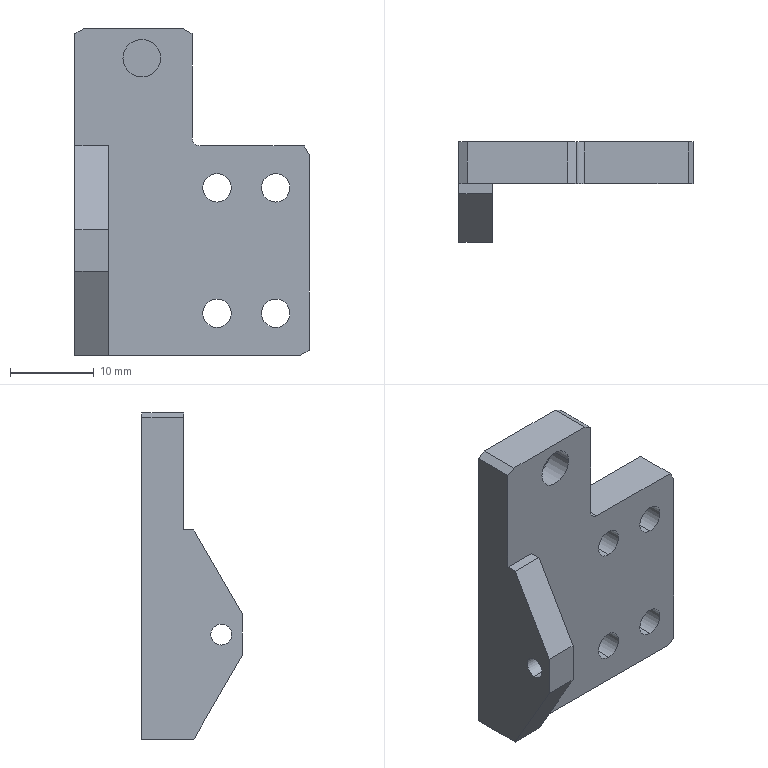Part | NX | features BREP 1 | 1 solid | 39 faces | box 28 x 12 x 39 mm | volume 4638 mm3 | plane 18 | cylinder 13 | cone 8 | commonest cylinder face diameters 3.4 x8 2.5 x2 4.5 x2 2 x1
STEP:
#1=CARTESIAN_POINT('',(14.,12.,13.5));
#2=VERTEX_POINT('',#1);
#3=CARTESIAN_POINT('',(15.,12.,12.5));
#4=VERTEX_POINT('',#3);
#5=CARTESIAN_POINT('',(15.,12.,13.5));
#6=DIRECTION('',(0.,-1.,0.));
#7=DIRECTION('',(0.,0.,-1.));
#8=AXIS2_PLACEMENT_3D('',#5,#6,#7);
#9=CIRCLE('',#8,1.);
#10=EDGE_CURVE('',#2,#4,#9,.T.);
#11=ORIENTED_EDGE('',*,*,#10,.F.);
#12=CARTESIAN_POINT('',(14.,7.,13.5));
#13=VERTEX_POINT('',#12);
#14=CARTESIAN_POINT('',(14.,12.,13.5));
#15=DIRECTION('',(0.,1.,0.));
#16=VECTOR('',#15,1000.);
#17=LINE('',#14,#16);
#18=EDGE_CURVE('',#13,#2,#17,.T.);
#19=ORIENTED_EDGE('',*,*,#18,.F.);
#20=CARTESIAN_POINT('',(15.,7.,12.5));
#21=VERTEX_POINT('',#20);
#22=CARTESIAN_POINT('',(15.,7.,13.5));
#23=DIRECTION('',(0.,1.,0.));
#24=DIRECTION('',(-1.,0.,0.));
#25=AXIS2_PLACEMENT_3D('',#22,#23,#24);
#26=CIRCLE('',#25,1.);
#27=EDGE_CURVE('',#21,#13,#26,.T.);
#28=ORIENTED_EDGE('',*,*,#27,.F.);
#29=CARTESIAN_POINT('',(15.,0.,12.5));
#30=DIRECTION('',(0.,-1.,0.));
#31=VECTOR('',#30,1000.);
#32=LINE('',#29,#31);
#33=EDGE_CURVE('',#4,#21,#32,.T.);
#34=ORIENTED_EDGE('',*,*,#33,.F.);
#35=EDGE_LOOP('',(#11,#19,#28,#34));
#36=FACE_BOUND('',#35,.T.);
#37=CARTESIAN_POINT('',(15.,0.,13.5));
#38=DIRECTION('',(0.,-1.,0.));
#39=DIRECTION('',(1.,0.,0.));
#40=AXIS2_PLACEMENT_3D('',#37,#38,#39);
#41=CYLINDRICAL_SURFACE('',#40,1.);
#42=ADVANCED_FACE('',(#36),#41,.F.);
#43=CARTESIAN_POINT('',(13.,12.,26.5));
#44=VERTEX_POINT('',#43);
#45=CARTESIAN_POINT('',(14.,12.,25.923));
#46=VERTEX_POINT('',#45);
#47=CARTESIAN_POINT('',(14.,12.,25.923));
#48=DIRECTION('',(0.866,0.,-0.5));
#49=VECTOR('',#48,1000.);
#50=LINE('',#47,#49);
#51=EDGE_CURVE('',#44,#46,#50,.T.);
#52=ORIENTED_EDGE('',*,*,#51,.F.);
#53=CARTESIAN_POINT('',(13.,7.,26.5));
#54=VERTEX_POINT('',#53);
#55=CARTESIAN_POINT('',(13.,0.,26.5));
#56=DIRECTION('',(0.,1.,0.));
#57=VECTOR('',#56,1000.);
#58=LINE('',#55,#57);
#59=EDGE_CURVE('',#54,#44,#58,.T.);
#60=ORIENTED_EDGE('',*,*,#59,.F.);
#61=CARTESIAN_POINT('',(14.,7.,25.923));
#62=VERTEX_POINT('',#61);
#63=CARTESIAN_POINT('',(14.,7.,25.923));
#64=DIRECTION('',(-0.866,0.,0.5));
#65=VECTOR('',#64,1000.);
#66=LINE('',#63,#65);
#67=EDGE_CURVE('',#62,#54,#66,.T.);
#68=ORIENTED_EDGE('',*,*,#67,.F.);
#69=CARTESIAN_POINT('',(14.,12.,25.923));
#70=DIRECTION('',(0.,-1.,0.));
#71=VECTOR('',#70,1000.);
#72=LINE('',#69,#71);
#73=EDGE_CURVE('',#46,#62,#72,.T.);
#74=ORIENTED_EDGE('',*,*,#73,.F.);
#75=EDGE_LOOP('',(#52,#60,#68,#74));
#76=FACE_BOUND('',#75,.T.);
#77=CARTESIAN_POINT('',(14.,12.,25.923));
#78=DIRECTION('',(-0.5,0.,-0.866));
#79=DIRECTION('',(0.,-1.,0.));
#80=AXIS2_PLACEMENT_3D('',#77,#78,#79);
#81=PLANE('',#80);
#82=ADVANCED_FACE('',(#76),#81,.F.);
#83=CARTESIAN_POINT('',(1.,7.,26.5));
#84=VERTEX_POINT('',#83);
#85=CARTESIAN_POINT('',(0.,7.,25.923));
#86=VERTEX_POINT('',#85);
#87=CARTESIAN_POINT('',(0.,7.,25.923));
#88=DIRECTION('',(-0.866,0.,-0.5));
#89=VECTOR('',#88,1000.);
#90=LINE('',#87,#89);
#91=EDGE_CURVE('',#84,#86,#90,.T.);
#92=ORIENTED_EDGE('',*,*,#91,.F.);
#93=CARTESIAN_POINT('',(1.,12.,26.5));
#94=VERTEX_POINT('',#93);
#95=CARTESIAN_POINT('',(1.,7.,26.5));
#96=DIRECTION('',(0.,-1.,0.));
#97=VECTOR('',#96,1000.);
#98=LINE('',#95,#97);
#99=EDGE_CURVE('',#94,#84,#98,.T.);
#100=ORIENTED_EDGE('',*,*,#99,.F.);
#101=CARTESIAN_POINT('',(0.,12.,25.923));
#102=VERTEX_POINT('',#101);
#103=CARTESIAN_POINT('',(0.,12.,25.923));
#104=DIRECTION('',(0.866,0.,0.5));
#105=VECTOR('',#104,1000.);
#106=LINE('',#103,#105);
#107=EDGE_CURVE('',#102,#94,#106,.T.);
#108=ORIENTED_EDGE('',*,*,#107,.F.);
#109=CARTESIAN_POINT('',(0.,12.,25.923));
#110=DIRECTION('',(0.,1.,0.));
#111=VECTOR('',#110,1000.);
#112=LINE('',#109,#111);
#113=EDGE_CURVE('',#86,#102,#112,.T.);
#114=ORIENTED_EDGE('',*,*,#113,.F.);
#115=EDGE_LOOP('',(#92,#100,#108,#114));
#116=FACE_BOUND('',#115,.T.);
#117=CARTESIAN_POINT('',(0.,0.,25.923));
#118=DIRECTION('',(-0.5,0.,0.866));
#119=DIRECTION('',(0.,-1.,0.));
#120=AXIS2_PLACEMENT_3D('',#117,#118,#119);
#121=PLANE('',#120);
#122=ADVANCED_FACE('',(#116),#121,.T.);
#123=CARTESIAN_POINT('',(27.,7.,-12.5));
#124=VERTEX_POINT('',#123);
#125=CARTESIAN_POINT('',(28.,7.,-11.923));
#126=VERTEX_POINT('',#125);
#127=CARTESIAN_POINT('',(28.,7.,-11.923));
#128=DIRECTION('',(0.866,0.,0.5));
#129=VECTOR('',#128,1000.);
#130=LINE('',#127,#129);
#131=EDGE_CURVE('',#124,#126,#130,.T.);
#132=ORIENTED_EDGE('',*,*,#131,.F.);
#133=CARTESIAN_POINT('',(27.,12.,-12.5));
#134=VERTEX_POINT('',#133);
#135=CARTESIAN_POINT('',(27.,7.,-12.5));
#136=DIRECTION('',(0.,-1.,0.));
#137=VECTOR('',#136,1000.);
#138=LINE('',#135,#137);
#139=EDGE_CURVE('',#134,#124,#138,.T.);
#140=ORIENTED_EDGE('',*,*,#139,.F.);
#141=CARTESIAN_POINT('',(28.,12.,-11.923));
#142=VERTEX_POINT('',#141);
#143=CARTESIAN_POINT('',(28.,12.,-11.923));
#144=DIRECTION('',(-0.866,0.,-0.5));
#145=VECTOR('',#144,1000.);
#146=LINE('',#143,#145);
#147=EDGE_CURVE('',#142,#134,#146,.T.);
#148=ORIENTED_EDGE('',*,*,#147,.F.);
#149=CARTESIAN_POINT('',(28.,12.,-11.923));
#150=DIRECTION('',(0.,1.,0.));
#151=VECTOR('',#150,1000.);
#152=LINE('',#149,#151);
#153=EDGE_CURVE('',#126,#142,#152,.T.);
#154=ORIENTED_EDGE('',*,*,#153,.F.);
#155=EDGE_LOOP('',(#132,#140,#148,#154));
#156=FACE_BOUND('',#155,.T.);
#157=CARTESIAN_POINT('',(28.,12.,-11.923));
#158=DIRECTION('',(0.5,0.,-0.866));
#159=DIRECTION('',(0.,-1.,0.));
#160=AXIS2_PLACEMENT_3D('',#157,#158,#159);
#161=PLANE('',#160);
#162=ADVANCED_FACE('',(#156),#161,.T.);
#163=CARTESIAN_POINT('',(28.,7.,11.5));
#164=VERTEX_POINT('',#163);
#165=CARTESIAN_POINT('',(27.423,7.,12.5));
#166=VERTEX_POINT('',#165);
#167=CARTESIAN_POINT('',(27.423,7.,12.5));
#168=DIRECTION('',(-0.5,0.,0.866));
#169=VECTOR('',#168,1000.);
#170=LINE('',#167,#169);
#171=EDGE_CURVE('',#164,#166,#170,.T.);
#172=ORIENTED_EDGE('',*,*,#171,.F.);
#173=CARTESIAN_POINT('',(28.,12.,11.5));
#174=VERTEX_POINT('',#173);
#175=CARTESIAN_POINT('',(28.,12.,11.5));
#176=DIRECTION('',(0.,-1.,0.));
#177=VECTOR('',#176,1000.);
#178=LINE('',#175,#177);
#179=EDGE_CURVE('',#174,#164,#178,.T.);
#180=ORIENTED_EDGE('',*,*,#179,.F.);
#181=CARTESIAN_POINT('',(27.423,12.,12.5));
#182=VERTEX_POINT('',#181);
#183=CARTESIAN_POINT('',(27.423,12.,12.5));
#184=DIRECTION('',(0.5,0.,-0.866));
#185=VECTOR('',#184,1000.);
#186=LINE('',#183,#185);
#187=EDGE_CURVE('',#182,#174,#186,.T.);
#188=ORIENTED_EDGE('',*,*,#187,.F.);
#189=CARTESIAN_POINT('',(27.423,0.,12.5));
#190=DIRECTION('',(0.,1.,0.));
#191=VECTOR('',#190,1000.);
#192=LINE('',#189,#191);
#193=EDGE_CURVE('',#166,#182,#192,.T.);
#194=ORIENTED_EDGE('',*,*,#193,.F.);
#195=EDGE_LOOP('',(#172,#180,#188,#194));
#196=FACE_BOUND('',#195,.T.);
#197=CARTESIAN_POINT('',(27.423,0.,12.5));
#198=DIRECTION('',(-0.866,0.,-0.5));
#199=DIRECTION('',(0.,1.,0.));
#200=AXIS2_PLACEMENT_3D('',#197,#198,#199);
#201=PLANE('',#200);
#202=ADVANCED_FACE('',(#196),#201,.F.);
#203=CARTESIAN_POINT('',(10.25,10.,23.));
#204=VERTEX_POINT('',#203);
#205=CARTESIAN_POINT('',(5.75,10.,23.));
#206=VERTEX_POINT('',#205);
#207=CARTESIAN_POINT('',(8.,10.,23.));
#208=DIRECTION('',(0.,-1.,0.));
#209=DIRECTION('',(1.,0.,0.));
#210=AXIS2_PLACEMENT_3D('',#207,#208,#209);
#211=CIRCLE('',#210,2.25);
#212=EDGE_CURVE('',#204,#206,#211,.T.);
#213=ORIENTED_EDGE('',*,*,#212,.T.);
#214=CARTESIAN_POINT('',(8.,10.,23.));
#215=DIRECTION('',(0.,-1.,0.));
#216=DIRECTION('',(1.,0.,0.));
#217=AXIS2_PLACEMENT_3D('',#214,#215,#216);
#218=CIRCLE('',#217,2.25);
#219=EDGE_CURVE('',#206,#204,#218,.T.);
#220=ORIENTED_EDGE('',*,*,#219,.T.);
#221=EDGE_LOOP('',(#213,#220));
#222=FACE_BOUND('',#221,.T.);
#223=CARTESIAN_POINT('',(8.,10.,23.));
#224=DIRECTION('',(0.,-1.,0.));
#225=DIRECTION('',(1.,0.,0.));
#226=AXIS2_PLACEMENT_3D('',#223,#224,#225);
#227=PLANE('',#226);
#228=ADVANCED_FACE('',(#222),#227,.T.);
#229=CARTESIAN_POINT('',(5.75,7.,23.));
#230=VERTEX_POINT('',#229);
#231=CARTESIAN_POINT('',(5.75,10.,23.));
#232=DIRECTION('',(0.,-1.,0.));
#233=VECTOR('',#232,1000.);
#234=LINE('',#231,#233);
#235=EDGE_CURVE('',#230,#206,#234,.F.);
#236=ORIENTED_EDGE('',*,*,#235,.T.);
#237=ORIENTED_EDGE('',*,*,#212,.F.);
#238=CARTESIAN_POINT('',(10.25,7.,23.));
#239=VERTEX_POINT('',#238);
#240=CARTESIAN_POINT('',(10.25,10.,23.));
#241=DIRECTION('',(0.,-1.,0.));
#242=VECTOR('',#241,1000.);
#243=LINE('',#240,#242);
#244=EDGE_CURVE('',#239,#204,#243,.F.);
#245=ORIENTED_EDGE('',*,*,#244,.F.);
#246=CARTESIAN_POINT('',(8.,7.,23.));
#247=DIRECTION('',(0.,-1.,0.));
#248=DIRECTION('',(1.,0.,0.));
#249=AXIS2_PLACEMENT_3D('',#246,#247,#248);
#250=CIRCLE('',#249,2.25);
#251=EDGE_CURVE('',#239,#230,#250,.T.);
#252=ORIENTED_EDGE('',*,*,#251,.T.);
#253=EDGE_LOOP('',(#236,#237,#245,#252));
#254=FACE_BOUND('',#253,.T.);
#255=CARTESIAN_POINT('',(8.,10.,23.));
#256=DIRECTION('',(0.,-1.,0.));
#257=DIRECTION('',(1.,0.,0.));
#258=AXIS2_PLACEMENT_3D('',#255,#256,#257);
#259=CYLINDRICAL_SURFACE('',#258,2.25);
#260=ADVANCED_FACE('',(#254),#259,.F.);
#261=CARTESIAN_POINT('',(0.,12.,26.5));
#262=DIRECTION('',(1.,0.,0.));
#263=VECTOR('',#262,1000.);
#264=LINE('',#261,#263);
#265=EDGE_CURVE('',#94,#44,#264,.T.);
#266=ORIENTED_EDGE('',*,*,#265,.F.);
#267=ORIENTED_EDGE('',*,*,#99,.T.);
#268=CARTESIAN_POINT('',(0.,7.,26.5));
#269=DIRECTION('',(-1.,0.,0.));
#270=VECTOR('',#269,1000.);
#271=LINE('',#268,#270);
#272=EDGE_CURVE('',#54,#84,#271,.T.);
#273=ORIENTED_EDGE('',*,*,#272,.F.);
#274=ORIENTED_EDGE('',*,*,#59,.T.);
#275=EDGE_LOOP('',(#266,#267,#273,#274));
#276=FACE_BOUND('',#275,.T.);
#277=CARTESIAN_POINT('',(0.,0.,26.5));
#278=DIRECTION('',(0.,0.,1.));
#279=DIRECTION('',(1.,0.,0.));
#280=AXIS2_PLACEMENT_3D('',#277,#278,#279);
#281=PLANE('',#280);
#282=ADVANCED_FACE('',(#276),#281,.T.);
#283=CARTESIAN_POINT('',(14.,7.,26.5));
#284=DIRECTION('',(0.,0.,-1.));
#285=VECTOR('',#284,1000.);
#286=LINE('',#283,#285);
#287=EDGE_CURVE('',#62,#13,#286,.T.);
#288=ORIENTED_EDGE('',*,*,#287,.T.);
#289=ORIENTED_EDGE('',*,*,#18,.T.);
#290=CARTESIAN_POINT('',(14.,12.,26.5));
#291=DIRECTION('',(0.,0.,-1.));
#292=VECTOR('',#291,1000.);
#293=LINE('',#290,#292);
#294=EDGE_CURVE('',#46,#2,#293,.T.);
#295=ORIENTED_EDGE('',*,*,#294,.F.);
#296=ORIENTED_EDGE('',*,*,#73,.T.);
#297=EDGE_LOOP('',(#288,#289,#295,#296));
#298=FACE_BOUND('',#297,.T.);
#299=CARTESIAN_POINT('',(14.,12.,26.5));
#300=DIRECTION('',(1.,0.,0.));
#301=DIRECTION('',(0.,1.,0.));
#302=AXIS2_PLACEMENT_3D('',#299,#300,#301);
#303=PLANE('',#302);
#304=ADVANCED_FACE('',(#298),#303,.T.);
#305=CARTESIAN_POINT('',(0.,0.,2.5));
#306=VERTEX_POINT('',#305);
#307=CARTESIAN_POINT('',(0.,5.774,12.5));
#308=VERTEX_POINT('',#307);
#309=CARTESIAN_POINT('',(0.,5.774,12.5));
#310=DIRECTION('',(0.,0.5,0.866));
#311=VECTOR('',#310,1000.);
#312=LINE('',#309,#311);
#313=EDGE_CURVE('',#306,#308,#312,.T.);
#314=ORIENTED_EDGE('',*,*,#313,.F.);
#315=CARTESIAN_POINT('',(4.,0.,2.5));
#316=VERTEX_POINT('',#315);
#317=CARTESIAN_POINT('',(4.,0.,2.5));
#318=DIRECTION('',(-1.,0.,0.));
#319=VECTOR('',#318,1000.);
#320=LINE('',#317,#319);
#321=EDGE_CURVE('',#316,#306,#320,.T.);
#322=ORIENTED_EDGE('',*,*,#321,.F.);
#323=CARTESIAN_POINT('',(4.,5.774,12.5));
#324=VERTEX_POINT('',#323);
#325=CARTESIAN_POINT('',(4.,5.774,12.5));
#326=DIRECTION('',(0.,-0.5,-0.866));
#327=VECTOR('',#326,1000.);
#328=LINE('',#325,#327);
#329=EDGE_CURVE('',#324,#316,#328,.T.);
#330=ORIENTED_EDGE('',*,*,#329,.F.);
#331=CARTESIAN_POINT('',(0.,5.774,12.5));
#332=DIRECTION('',(1.,0.,0.));
#333=VECTOR('',#332,1000.);
#334=LINE('',#331,#333);
#335=EDGE_CURVE('',#308,#324,#334,.T.);
#336=ORIENTED_EDGE('',*,*,#335,.F.);
#337=EDGE_LOOP('',(#314,#322,#330,#336));
#338=FACE_BOUND('',#337,.T.);
#339=CARTESIAN_POINT('',(0.,5.774,12.5));
#340=DIRECTION('',(0.,0.866,-0.5));
#341=DIRECTION('',(1.,0.,0.));
#342=AXIS2_PLACEMENT_3D('',#339,#340,#341);
#343=PLANE('',#342);
#344=ADVANCED_FACE('',(#338),#343,.F.);
#345=CARTESIAN_POINT('',(0.,5.774,-12.5));
#346=VERTEX_POINT('',#345);
#347=CARTESIAN_POINT('',(0.,0.,-2.5));
#348=VERTEX_POINT('',#347);
#349=CARTESIAN_POINT('',(0.,0.,-2.5));
#350=DIRECTION('',(0.,-0.5,0.866));
#351=VECTOR('',#350,1000.);
#352=LINE('',#349,#351);
#353=EDGE_CURVE('',#346,#348,#352,.T.);
#354=ORIENTED_EDGE('',*,*,#353,.F.);
#355=CARTESIAN_POINT('',(4.,5.774,-12.5));
#356=VERTEX_POINT('',#355);
#357=CARTESIAN_POINT('',(0.,5.774,-12.5));
#358=DIRECTION('',(-1.,0.,0.));
#359=VECTOR('',#358,1000.);
#360=LINE('',#357,#359);
#361=EDGE_CURVE('',#356,#346,#360,.T.);
#362=ORIENTED_EDGE('',*,*,#361,.F.);
#363=CARTESIAN_POINT('',(4.,0.,-2.5));
#364=VERTEX_POINT('',#363);
#365=CARTESIAN_POINT('',(4.,0.,-2.5));
#366=DIRECTION('',(0.,0.5,-0.866));
#367=VECTOR('',#366,1000.);
#368=LINE('',#365,#367);
#369=EDGE_CURVE('',#364,#356,#368,.T.);
#370=ORIENTED_EDGE('',*,*,#369,.F.);
#371=CARTESIAN_POINT('',(4.,0.,-2.5));
#372=DIRECTION('',(1.,0.,0.));
#373=VECTOR('',#372,1000.);
#374=LINE('',#371,#373);
#375=EDGE_CURVE('',#348,#364,#374,.T.);
#376=ORIENTED_EDGE('',*,*,#375,.F.);
#377=EDGE_LOOP('',(#354,#362,#370,#376));
#378=FACE_BOUND('',#377,.T.);
#379=CARTESIAN_POINT('',(4.,0.,-2.5));
#380=DIRECTION('',(0.,-0.866,-0.5));
#381=DIRECTION('',(-1.,0.,0.));
#382=AXIS2_PLACEMENT_3D('',#379,#380,#381);
#383=PLANE('',#382);
#384=ADVANCED_FACE('',(#378),#383,.T.);
#385=CARTESIAN_POINT('',(17.,12.,4.35));
#386=VERTEX_POINT('',#385);
#387=CARTESIAN_POINT('',(17.,10.55,5.8));
#388=VERTEX_POINT('',#387);
#389=CARTESIAN_POINT('',(17.,12.,4.35));
#390=DIRECTION('',(0.,0.7071,-0.7071));
#391=VECTOR('',#390,1000.);
#392=LINE('',#389,#391);
#393=EDGE_CURVE('',#386,#388,#392,.F.);
#394=ORIENTED_EDGE('',*,*,#393,.T.);
#395=CARTESIAN_POINT('',(17.,10.55,9.2));
#396=VERTEX_POINT('',#395);
#397=CARTESIAN_POINT('',(17.,10.55,7.5));
#398=DIRECTION('',(0.,1.,0.));
#399=DIRECTION('',(0.,0.,1.));
#400=AXIS2_PLACEMENT_3D('',#397,#398,#399);
#401=CIRCLE('',#400,1.7);
#402=EDGE_CURVE('',#396,#388,#401,.T.);
#403=ORIENTED_EDGE('',*,*,#402,.F.);
#404=CARTESIAN_POINT('',(17.,12.,10.65));
#405=VERTEX_POINT('',#404);
#406=CARTESIAN_POINT('',(17.,12.,10.65));
#407=DIRECTION('',(0.,0.7071,0.7071));
#408=VECTOR('',#407,1000.);
#409=LINE('',#406,#408);
#410=EDGE_CURVE('',#405,#396,#409,.F.);
#411=ORIENTED_EDGE('',*,*,#410,.F.);
#412=CARTESIAN_POINT('',(17.,12.,7.5));
#413=DIRECTION('',(0.,1.,0.));
#414=DIRECTION('',(0.,0.,1.));
#415=AXIS2_PLACEMENT_3D('',#412,#413,#414);
#416=CIRCLE('',#415,3.15);
#417=EDGE_CURVE('',#405,#386,#416,.T.);
#418=ORIENTED_EDGE('',*,*,#417,.T.);
#419=EDGE_LOOP('',(#394,#403,#411,#418));
#420=FACE_BOUND('',#419,.T.);
#421=CARTESIAN_POINT('',(17.,12.,7.5));
#422=DIRECTION('',(0.,1.,0.));
#423=DIRECTION('',(0.,0.,1.));
#424=AXIS2_PLACEMENT_3D('',#421,#422,#423);
#425=CONICAL_SURFACE('',#424,3.15,0.7854);
#426=ADVANCED_FACE('',(#420),#425,.F.);
#427=CARTESIAN_POINT('',(17.,7.,5.8));
#428=VERTEX_POINT('',#427);
#429=CARTESIAN_POINT('',(17.,12.,5.8));
#430=DIRECTION('',(0.,1.,0.));
#431=VECTOR('',#430,1000.);
#432=LINE('',#429,#431);
#433=EDGE_CURVE('',#388,#428,#432,.F.);
#434=ORIENTED_EDGE('',*,*,#433,.T.);
#435=CARTESIAN_POINT('',(17.,7.,9.2));
#436=VERTEX_POINT('',#435);
#437=CARTESIAN_POINT('',(17.,7.,7.5));
#438=DIRECTION('',(0.,1.,0.));
#439=DIRECTION('',(-1.,0.,0.));
#440=AXIS2_PLACEMENT_3D('',#437,#438,#439);
#441=CIRCLE('',#440,1.7);
#442=EDGE_CURVE('',#436,#428,#441,.T.);
#443=ORIENTED_EDGE('',*,*,#442,.F.);
#444=CARTESIAN_POINT('',(17.,12.,9.2));
#445=DIRECTION('',(0.,1.,0.));
#446=VECTOR('',#445,1000.);
#447=LINE('',#444,#446);
#448=EDGE_CURVE('',#396,#436,#447,.F.);
#449=ORIENTED_EDGE('',*,*,#448,.F.);
#450=ORIENTED_EDGE('',*,*,#402,.T.);
#451=EDGE_LOOP('',(#434,#443,#449,#450));
#452=FACE_BOUND('',#451,.T.);
#453=CARTESIAN_POINT('',(17.,12.,7.5));
#454=DIRECTION('',(0.,1.,0.));
#455=DIRECTION('',(0.,0.,1.));
#456=AXIS2_PLACEMENT_3D('',#453,#454,#455);
#457=CYLINDRICAL_SURFACE('',#456,1.7);
#458=ADVANCED_FACE('',(#452),#457,.F.);
#459=CARTESIAN_POINT('',(24.,12.,4.35));
#460=VERTEX_POINT('',#459);
#461=CARTESIAN_POINT('',(24.,10.55,5.8));
#462=VERTEX_POINT('',#461);
#463=CARTESIAN_POINT('',(24.,12.,4.35));
#464=DIRECTION('',(0.,0.7071,-0.7071));
#465=VECTOR('',#464,1000.);
#466=LINE('',#463,#465);
#467=EDGE_CURVE('',#460,#462,#466,.F.);
#468=ORIENTED_EDGE('',*,*,#467,.T.);
#469=CARTESIAN_POINT('',(24.,10.55,9.2));
#470=VERTEX_POINT('',#469);
#471=CARTESIAN_POINT('',(24.,10.55,7.5));
#472=DIRECTION('',(0.,1.,0.));
#473=DIRECTION('',(0.,0.,1.));
#474=AXIS2_PLACEMENT_3D('',#471,#472,#473);
#475=CIRCLE('',#474,1.7);
#476=EDGE_CURVE('',#470,#462,#475,.T.);
#477=ORIENTED_EDGE('',*,*,#476,.F.);
#478=CARTESIAN_POINT('',(24.,12.,10.65));
#479=VERTEX_POINT('',#478);
#480=CARTESIAN_POINT('',(24.,12.,10.65));
#481=DIRECTION('',(0.,0.7071,0.7071));
#482=VECTOR('',#481,1000.);
#483=LINE('',#480,#482);
#484=EDGE_CURVE('',#479,#470,#483,.F.);
#485=ORIENTED_EDGE('',*,*,#484,.F.);
#486=CARTESIAN_POINT('',(24.,12.,7.5));
#487=DIRECTION('',(0.,1.,0.));
#488=DIRECTION('',(0.,0.,1.));
#489=AXIS2_PLACEMENT_3D('',#486,#487,#488);
#490=CIRCLE('',#489,3.15);
#491=EDGE_CURVE('',#479,#460,#490,.T.);
#492=ORIENTED_EDGE('',*,*,#491,.T.);
#493=EDGE_LOOP('',(#468,#477,#485,#492));
#494=FACE_BOUND('',#493,.T.);
#495=CARTESIAN_POINT('',(24.,12.,7.5));
#496=DIRECTION('',(0.,1.,0.));
#497=DIRECTION('',(0.,0.,1.));
#498=AXIS2_PLACEMENT_3D('',#495,#496,#497);
#499=CONICAL_SURFACE('',#498,3.15,0.7854);
#500=ADVANCED_FACE('',(#494),#499,.F.);
#501=CARTESIAN_POINT('',(24.,7.,5.8));
#502=VERTEX_POINT('',#501);
#503=CARTESIAN_POINT('',(24.,12.,5.8));
#504=DIRECTION('',(0.,1.,0.));
#505=VECTOR('',#504,1000.);
#506=LINE('',#503,#505);
#507=EDGE_CURVE('',#462,#502,#506,.F.);
#508=ORIENTED_EDGE('',*,*,#507,.T.);
#509=CARTESIAN_POINT('',(24.,7.,9.2));
#510=VERTEX_POINT('',#509);
#511=CARTESIAN_POINT('',(24.,7.,7.5));
#512=DIRECTION('',(0.,1.,0.));
#513=DIRECTION('',(-1.,0.,0.));
#514=AXIS2_PLACEMENT_3D('',#511,#512,#513);
#515=CIRCLE('',#514,1.7);
#516=EDGE_CURVE('',#510,#502,#515,.T.);
#517=ORIENTED_EDGE('',*,*,#516,.F.);
#518=CARTESIAN_POINT('',(24.,12.,9.2));
#519=DIRECTION('',(0.,1.,0.));
#520=VECTOR('',#519,1000.);
#521=LINE('',#518,#520);
#522=EDGE_CURVE('',#470,#510,#521,.F.);
#523=ORIENTED_EDGE('',*,*,#522,.F.);
#524=ORIENTED_EDGE('',*,*,#476,.T.);
#525=EDGE_LOOP('',(#508,#517,#523,#524));
#526=FACE_BOUND('',#525,.T.);
#527=CARTESIAN_POINT('',(24.,12.,7.5));
#528=DIRECTION('',(0.,1.,0.));
#529=DIRECTION('',(0.,0.,1.));
#530=AXIS2_PLACEMENT_3D('',#527,#528,#529);
#531=CYLINDRICAL_SURFACE('',#530,1.7);
#532=ADVANCED_FACE('',(#526),#531,.F.);
#533=CARTESIAN_POINT('',(17.,12.,-10.65));
#534=VERTEX_POINT('',#533);
#535=CARTESIAN_POINT('',(17.,10.55,-9.2));
#536=VERTEX_POINT('',#535);
#537=CARTESIAN_POINT('',(17.,12.,-10.65));
#538=DIRECTION('',(0.,0.7071,-0.7071));
#539=VECTOR('',#538,1000.);
#540=LINE('',#537,#539);
#541=EDGE_CURVE('',#534,#536,#540,.F.);
#542=ORIENTED_EDGE('',*,*,#541,.T.);
#543=CARTESIAN_POINT('',(17.,10.55,-5.8));
#544=VERTEX_POINT('',#543);
#545=CARTESIAN_POINT('',(17.,10.55,-7.5));
#546=DIRECTION('',(0.,1.,0.));
#547=DIRECTION('',(0.,0.,1.));
#548=AXIS2_PLACEMENT_3D('',#545,#546,#547);
#549=CIRCLE('',#548,1.7);
#550=EDGE_CURVE('',#544,#536,#549,.T.);
#551=ORIENTED_EDGE('',*,*,#550,.F.);
#552=CARTESIAN_POINT('',(17.,12.,-4.35));
#553=VERTEX_POINT('',#552);
#554=CARTESIAN_POINT('',(17.,12.,-4.35));
#555=DIRECTION('',(0.,0.7071,0.7071));
#556=VECTOR('',#555,1000.);
#557=LINE('',#554,#556);
#558=EDGE_CURVE('',#553,#544,#557,.F.);
#559=ORIENTED_EDGE('',*,*,#558,.F.);
#560=CARTESIAN_POINT('',(17.,12.,-7.5));
#561=DIRECTION('',(0.,1.,0.));
#562=DIRECTION('',(0.,0.,1.));
#563=AXIS2_PLACEMENT_3D('',#560,#561,#562);
#564=CIRCLE('',#563,3.15);
#565=EDGE_CURVE('',#553,#534,#564,.T.);
#566=ORIENTED_EDGE('',*,*,#565,.T.);
#567=EDGE_LOOP('',(#542,#551,#559,#566));
#568=FACE_BOUND('',#567,.T.);
#569=CARTESIAN_POINT('',(17.,12.,-7.5));
#570=DIRECTION('',(0.,1.,0.));
#571=DIRECTION('',(0.,0.,1.));
#572=AXIS2_PLACEMENT_3D('',#569,#570,#571);
#573=CONICAL_SURFACE('',#572,3.15,0.7854);
#574=ADVANCED_FACE('',(#568),#573,.F.);
#575=CARTESIAN_POINT('',(17.,7.,-9.2));
#576=VERTEX_POINT('',#575);
#577=CARTESIAN_POINT('',(17.,12.,-9.2));
#578=DIRECTION('',(0.,1.,0.));
#579=VECTOR('',#578,1000.);
#580=LINE('',#577,#579);
#581=EDGE_CURVE('',#536,#576,#580,.F.);
#582=ORIENTED_EDGE('',*,*,#581,.T.);
#583=CARTESIAN_POINT('',(17.,7.,-5.8));
#584=VERTEX_POINT('',#583);
#585=CARTESIAN_POINT('',(17.,7.,-7.5));
#586=DIRECTION('',(0.,1.,0.));
#587=DIRECTION('',(-1.,0.,0.));
#588=AXIS2_PLACEMENT_3D('',#585,#586,#587);
#589=CIRCLE('',#588,1.7);
#590=EDGE_CURVE('',#584,#576,#589,.T.);
#591=ORIENTED_EDGE('',*,*,#590,.F.);
#592=CARTESIAN_POINT('',(17.,12.,-5.8));
#593=DIRECTION('',(0.,1.,0.));
#594=VECTOR('',#593,1000.);
#595=LINE('',#592,#594);
#596=EDGE_CURVE('',#544,#584,#595,.F.);
#597=ORIENTED_EDGE('',*,*,#596,.F.);
#598=ORIENTED_EDGE('',*,*,#550,.T.);
#599=EDGE_LOOP('',(#582,#591,#597,#598));
#600=FACE_BOUND('',#599,.T.);
#601=CARTESIAN_POINT('',(17.,12.,-7.5));
#602=DIRECTION('',(0.,1.,0.));
#603=DIRECTION('',(0.,0.,1.));
#604=AXIS2_PLACEMENT_3D('',#601,#602,#603);
#605=CYLINDRICAL_SURFACE('',#604,1.7);
#606=ADVANCED_FACE('',(#600),#605,.F.);
#607=CARTESIAN_POINT('',(24.,12.,-10.65));
#608=VERTEX_POINT('',#607);
#609=CARTESIAN_POINT('',(24.,10.55,-9.2));
#610=VERTEX_POINT('',#609);
#611=CARTESIAN_POINT('',(24.,12.,-10.65));
#612=DIRECTION('',(0.,0.7071,-0.7071));
#613=VECTOR('',#612,1000.);
#614=LINE('',#611,#613);
#615=EDGE_CURVE('',#608,#610,#614,.F.);
#616=ORIENTED_EDGE('',*,*,#615,.T.);
#617=CARTESIAN_POINT('',(24.,10.55,-5.8));
#618=VERTEX_POINT('',#617);
#619=CARTESIAN_POINT('',(24.,10.55,-7.5));
#620=DIRECTION('',(0.,1.,0.));
#621=DIRECTION('',(0.,0.,1.));
#622=AXIS2_PLACEMENT_3D('',#619,#620,#621);
#623=CIRCLE('',#622,1.7);
#624=EDGE_CURVE('',#618,#610,#623,.T.);
#625=ORIENTED_EDGE('',*,*,#624,.F.);
#626=CARTESIAN_POINT('',(24.,12.,-4.35));
#627=VERTEX_POINT('',#626);
#628=CARTESIAN_POINT('',(24.,12.,-4.35));
#629=DIRECTION('',(0.,0.7071,0.7071));
#630=VECTOR('',#629,1000.);
#631=LINE('',#628,#630);
#632=EDGE_CURVE('',#627,#618,#631,.F.);
#633=ORIENTED_EDGE('',*,*,#632,.F.);
#634=CARTESIAN_POINT('',(24.,12.,-7.5));
#635=DIRECTION('',(0.,1.,0.));
#636=DIRECTION('',(0.,0.,1.));
#637=AXIS2_PLACEMENT_3D('',#634,#635,#636);
#638=CIRCLE('',#637,3.15);
#639=EDGE_CURVE('',#627,#608,#638,.T.);
#640=ORIENTED_EDGE('',*,*,#639,.T.);
#641=EDGE_LOOP('',(#616,#625,#633,#640));
#642=FACE_BOUND('',#641,.T.);
#643=CARTESIAN_POINT('',(24.,12.,-7.5));
#644=DIRECTION('',(0.,1.,0.));
#645=DIRECTION('',(0.,0.,1.));
#646=AXIS2_PLACEMENT_3D('',#643,#644,#645);
#647=CONICAL_SURFACE('',#646,3.15,0.7854);
#648=ADVANCED_FACE('',(#642),#647,.F.);
#649=CARTESIAN_POINT('',(24.,7.,-9.2));
#650=VERTEX_POINT('',#649);
#651=CARTESIAN_POINT('',(24.,12.,-9.2));
#652=DIRECTION('',(0.,1.,0.));
#653=VECTOR('',#652,1000.);
#654=LINE('',#651,#653);
#655=EDGE_CURVE('',#610,#650,#654,.F.);
#656=ORIENTED_EDGE('',*,*,#655,.T.);
#657=CARTESIAN_POINT('',(24.,7.,-5.8));
#658=VERTEX_POINT('',#657);
#659=CARTESIAN_POINT('',(24.,7.,-7.5));
#660=DIRECTION('',(0.,1.,0.));
#661=DIRECTION('',(-1.,0.,0.));
#662=AXIS2_PLACEMENT_3D('',#659,#660,#661);
#663=CIRCLE('',#662,1.7);
#664=EDGE_CURVE('',#658,#650,#663,.T.);
#665=ORIENTED_EDGE('',*,*,#664,.F.);
#666=CARTESIAN_POINT('',(24.,12.,-5.8));
#667=DIRECTION('',(0.,1.,0.));
#668=VECTOR('',#667,1000.);
#669=LINE('',#666,#668);
#670=EDGE_CURVE('',#618,#658,#669,.F.);
#671=ORIENTED_EDGE('',*,*,#670,.F.);
#672=ORIENTED_EDGE('',*,*,#624,.T.);
#673=EDGE_LOOP('',(#656,#665,#671,#672));
#674=FACE_BOUND('',#673,.T.);
#675=CARTESIAN_POINT('',(24.,12.,-7.5));
#676=DIRECTION('',(0.,1.,0.));
#677=DIRECTION('',(0.,0.,1.));
#678=AXIS2_PLACEMENT_3D('',#675,#676,#677);
#679=CYLINDRICAL_SURFACE('',#678,1.7);
#680=ADVANCED_FACE('',(#674),#679,.F.);
#681=CARTESIAN_POINT('',(0.,2.5,-1.25));
#682=VERTEX_POINT('',#681);
#683=CARTESIAN_POINT('',(4.,2.5,-1.25));
#684=VERTEX_POINT('',#683);
#685=CARTESIAN_POINT('',(0.,2.5,-1.25));
#686=DIRECTION('',(-1.,0.,0.));
#687=VECTOR('',#686,1000.);
#688=LINE('',#685,#687);
#689=EDGE_CURVE('',#682,#684,#688,.F.);
#690=ORIENTED_EDGE('',*,*,#689,.T.);
#691=CARTESIAN_POINT('',(4.,2.5,1.25));
#692=VERTEX_POINT('',#691);
#693=CARTESIAN_POINT('',(4.,2.5,0.));
#694=DIRECTION('',(-1.,0.,0.));
#695=DIRECTION('',(0.,0.,1.));
#696=AXIS2_PLACEMENT_3D('',#693,#694,#695);
#697=CIRCLE('',#696,1.25);
#698=EDGE_CURVE('',#692,#684,#697,.T.);
#699=ORIENTED_EDGE('',*,*,#698,.F.);
#700=CARTESIAN_POINT('',(0.,2.5,1.25));
#701=VERTEX_POINT('',#700);
#702=CARTESIAN_POINT('',(0.,2.5,1.25));
#703=DIRECTION('',(-1.,0.,0.));
#704=VECTOR('',#703,1000.);
#705=LINE('',#702,#704);
#706=EDGE_CURVE('',#701,#692,#705,.F.);
#707=ORIENTED_EDGE('',*,*,#706,.F.);
#708=CARTESIAN_POINT('',(0.,2.5,0.));
#709=DIRECTION('',(-1.,0.,0.));
#710=DIRECTION('',(0.,0.,1.));
#711=AXIS2_PLACEMENT_3D('',#708,#709,#710);
#712=CIRCLE('',#711,1.25);
#713=EDGE_CURVE('',#701,#682,#712,.T.);
#714=ORIENTED_EDGE('',*,*,#713,.T.);
#715=EDGE_LOOP('',(#690,#699,#707,#714));
#716=FACE_BOUND('',#715,.T.);
#717=CARTESIAN_POINT('',(0.,2.5,0.));
#718=DIRECTION('',(-1.,0.,0.));
#719=DIRECTION('',(0.,0.,1.));
#720=AXIS2_PLACEMENT_3D('',#717,#718,#719);
#721=CYLINDRICAL_SURFACE('',#720,1.25);
#722=ADVANCED_FACE('',(#716),#721,.F.);
#723=CARTESIAN_POINT('',(0.,12.,-12.5));
#724=VERTEX_POINT('',#723);
#725=CARTESIAN_POINT('',(0.,12.,-12.5));
#726=DIRECTION('',(-1.,0.,0.));
#727=VECTOR('',#726,1000.);
#728=LINE('',#725,#727);
#729=EDGE_CURVE('',#134,#724,#728,.T.);
#730=ORIENTED_EDGE('',*,*,#729,.F.);
#731=ORIENTED_EDGE('',*,*,#139,.T.);
#732=CARTESIAN_POINT('',(4.,7.,-12.5));
#733=VERTEX_POINT('',#732);
#734=CARTESIAN_POINT('',(28.,7.,-12.5));
#735=DIRECTION('',(1.,0.,0.));
#736=VECTOR('',#735,1000.);
#737=LINE('',#734,#736);
#738=EDGE_CURVE('',#733,#124,#737,.T.);
#739=ORIENTED_EDGE('',*,*,#738,.F.);
#740=CARTESIAN_POINT('',(4.,7.,-12.5));
#741=DIRECTION('',(0.,1.,0.));
#742=VECTOR('',#741,1000.);
#743=LINE('',#740,#742);
#744=EDGE_CURVE('',#356,#733,#743,.T.);
#745=ORIENTED_EDGE('',*,*,#744,.F.);
#746=ORIENTED_EDGE('',*,*,#361,.T.);
#747=CARTESIAN_POINT('',(0.,0.,-12.5));
#748=DIRECTION('',(0.,-1.,0.));
#749=VECTOR('',#748,1000.);
#750=LINE('',#747,#749);
#751=EDGE_CURVE('',#724,#346,#750,.T.);
#752=ORIENTED_EDGE('',*,*,#751,.F.);
#753=EDGE_LOOP('',(#730,#731,#739,#745,#746,#752));
#754=FACE_BOUND('',#753,.T.);
#755=CARTESIAN_POINT('',(0.,0.,-12.5));
#756=DIRECTION('',(0.,0.,-1.));
#757=DIRECTION('',(-1.,0.,0.));
#758=AXIS2_PLACEMENT_3D('',#755,#756,#757);
#759=PLANE('',#758);
#760=ADVANCED_FACE('',(#754),#759,.T.);
#761=CARTESIAN_POINT('',(4.,7.,12.5));
#762=VERTEX_POINT('',#761);
#763=CARTESIAN_POINT('',(4.,7.,12.5));
#764=DIRECTION('',(0.,1.,0.));
#765=VECTOR('',#764,1000.);
#766=LINE('',#763,#765);
#767=EDGE_CURVE('',#324,#762,#766,.T.);
#768=ORIENTED_EDGE('',*,*,#767,.T.);
#769=CARTESIAN_POINT('',(0.,7.,12.5));
#770=VERTEX_POINT('',#769);
#771=CARTESIAN_POINT('',(0.,7.,12.5));
#772=DIRECTION('',(-1.,0.,0.));
#773=VECTOR('',#772,1000.);
#774=LINE('',#771,#773);
#775=EDGE_CURVE('',#762,#770,#774,.T.);
#776=ORIENTED_EDGE('',*,*,#775,.T.);
#777=CARTESIAN_POINT('',(0.,0.,12.5));
#778=DIRECTION('',(0.,-1.,0.));
#779=VECTOR('',#778,1000.);
#780=LINE('',#777,#779);
#781=EDGE_CURVE('',#770,#308,#780,.T.);
#782=ORIENTED_EDGE('',*,*,#781,.T.);
#783=ORIENTED_EDGE('',*,*,#335,.T.);
#784=EDGE_LOOP('',(#768,#776,#782,#783));
#785=FACE_BOUND('',#784,.T.);
#786=CARTESIAN_POINT('',(0.,0.,12.5));
#787=DIRECTION('',(0.,0.,-1.));
#788=DIRECTION('',(-1.,0.,0.));
#789=AXIS2_PLACEMENT_3D('',#786,#787,#788);
#790=PLANE('',#789);
#791=ADVANCED_FACE('',(#785),#790,.F.);
#792=CARTESIAN_POINT('',(0.,7.,26.5));
#793=DIRECTION('',(0.,0.,-1.));
#794=VECTOR('',#793,1000.);
#795=LINE('',#792,#794);
#796=EDGE_CURVE('',#86,#770,#795,.T.);
#797=ORIENTED_EDGE('',*,*,#796,.F.);
#798=ORIENTED_EDGE('',*,*,#113,.T.);
#799=CARTESIAN_POINT('',(0.,12.,12.5));
#800=DIRECTION('',(0.,0.,-1.));
#801=VECTOR('',#800,1000.);
#802=LINE('',#799,#801);
#803=EDGE_CURVE('',#102,#724,#802,.T.);
#804=ORIENTED_EDGE('',*,*,#803,.T.);
#805=ORIENTED_EDGE('',*,*,#751,.T.);
#806=ORIENTED_EDGE('',*,*,#353,.T.);
#807=CARTESIAN_POINT('',(0.,0.,12.5));
#808=DIRECTION('',(0.,0.,-1.));
#809=VECTOR('',#808,1000.);
#810=LINE('',#807,#809);
#811=EDGE_CURVE('',#306,#348,#810,.T.);
#812=ORIENTED_EDGE('',*,*,#811,.F.);
#813=ORIENTED_EDGE('',*,*,#313,.T.);
#814=ORIENTED_EDGE('',*,*,#781,.F.);
#815=EDGE_LOOP('',(#797,#798,#804,#805,#806,#812,#813,#814));
#816=FACE_BOUND('',#815,.T.);
#817=ORIENTED_EDGE('',*,*,#713,.F.);
#818=CARTESIAN_POINT('',(0.,2.5,0.));
#819=DIRECTION('',(-1.,0.,0.));
#820=DIRECTION('',(0.,0.,1.));
#821=AXIS2_PLACEMENT_3D('',#818,#819,#820);
#822=CIRCLE('',#821,1.25);
#823=EDGE_CURVE('',#682,#701,#822,.T.);
#824=ORIENTED_EDGE('',*,*,#823,.F.);
#825=EDGE_LOOP('',(#817,#824));
#826=FACE_BOUND('',#825,.T.);
#827=CARTESIAN_POINT('',(0.,0.,12.5));
#828=DIRECTION('',(1.,0.,0.));
#829=DIRECTION('',(0.,0.,-1.));
#830=AXIS2_PLACEMENT_3D('',#827,#828,#829);
#831=PLANE('',#830);
#832=ADVANCED_FACE('',(#816,#826),#831,.F.);
#833=CARTESIAN_POINT('',(0.,12.,12.5));
#834=DIRECTION('',(-1.,0.,0.));
#835=VECTOR('',#834,1000.);
#836=LINE('',#833,#835);
#837=EDGE_CURVE('',#182,#4,#836,.T.);
#838=ORIENTED_EDGE('',*,*,#837,.F.);
#839=ORIENTED_EDGE('',*,*,#187,.T.);
#840=CARTESIAN_POINT('',(28.,12.,12.5));
#841=DIRECTION('',(0.,0.,-1.));
#842=VECTOR('',#841,1000.);
#843=LINE('',#840,#842);
#844=EDGE_CURVE('',#174,#142,#843,.T.);
#845=ORIENTED_EDGE('',*,*,#844,.T.);
#846=ORIENTED_EDGE('',*,*,#147,.T.);
#847=ORIENTED_EDGE('',*,*,#729,.T.);
#848=ORIENTED_EDGE('',*,*,#803,.F.);
#849=ORIENTED_EDGE('',*,*,#107,.T.);
#850=ORIENTED_EDGE('',*,*,#265,.T.);
#851=ORIENTED_EDGE('',*,*,#51,.T.);
#852=ORIENTED_EDGE('',*,*,#294,.T.);
#853=ORIENTED_EDGE('',*,*,#10,.T.);
#854=EDGE_LOOP('',(#838,#839,#845,#846,#847,#848,#849,#850,#851,#852,#853));
#855=FACE_BOUND('',#854,.T.);
#856=ORIENTED_EDGE('',*,*,#639,.F.);
#857=CARTESIAN_POINT('',(24.,12.,-7.5));
#858=DIRECTION('',(0.,1.,0.));
#859=DIRECTION('',(0.,0.,1.));
#860=AXIS2_PLACEMENT_3D('',#857,#858,#859);
#861=CIRCLE('',#860,3.15);
#862=EDGE_CURVE('',#608,#627,#861,.T.);
#863=ORIENTED_EDGE('',*,*,#862,.F.);
#864=EDGE_LOOP('',(#856,#863));
#865=FACE_BOUND('',#864,.T.);
#866=ORIENTED_EDGE('',*,*,#565,.F.);
#867=CARTESIAN_POINT('',(17.,12.,-7.5));
#868=DIRECTION('',(0.,1.,0.));
#869=DIRECTION('',(0.,0.,1.));
#870=AXIS2_PLACEMENT_3D('',#867,#868,#869);
#871=CIRCLE('',#870,3.15);
#872=EDGE_CURVE('',#534,#553,#871,.T.);
#873=ORIENTED_EDGE('',*,*,#872,.F.);
#874=EDGE_LOOP('',(#866,#873));
#875=FACE_BOUND('',#874,.T.);
#876=ORIENTED_EDGE('',*,*,#491,.F.);
#877=CARTESIAN_POINT('',(24.,12.,7.5));
#878=DIRECTION('',(0.,1.,0.));
#879=DIRECTION('',(0.,0.,1.));
#880=AXIS2_PLACEMENT_3D('',#877,#878,#879);
#881=CIRCLE('',#880,3.15);
#882=EDGE_CURVE('',#460,#479,#881,.T.);
#883=ORIENTED_EDGE('',*,*,#882,.F.);
#884=EDGE_LOOP('',(#876,#883));
#885=FACE_BOUND('',#884,.T.);
#886=ORIENTED_EDGE('',*,*,#417,.F.);
#887=CARTESIAN_POINT('',(17.,12.,7.5));
#888=DIRECTION('',(0.,1.,0.));
#889=DIRECTION('',(0.,0.,1.));
#890=AXIS2_PLACEMENT_3D('',#887,#888,#889);
#891=CIRCLE('',#890,3.15);
#892=EDGE_CURVE('',#386,#405,#891,.T.);
#893=ORIENTED_EDGE('',*,*,#892,.F.);
#894=EDGE_LOOP('',(#886,#893));
#895=FACE_BOUND('',#894,.T.);
#896=CARTESIAN_POINT('',(0.,12.,12.5));
#897=DIRECTION('',(0.,-1.,0.));
#898=DIRECTION('',(0.,0.,-1.));
#899=AXIS2_PLACEMENT_3D('',#896,#897,#898);
#900=PLANE('',#899);
#901=ADVANCED_FACE('',(#855,#865,#875,#885,#895),#900,.F.);
#902=ORIENTED_EDGE('',*,*,#844,.F.);
#903=ORIENTED_EDGE('',*,*,#179,.T.);
#904=CARTESIAN_POINT('',(28.,7.,12.5));
#905=DIRECTION('',(0.,0.,-1.));
#906=VECTOR('',#905,1000.);
#907=LINE('',#904,#906);
#908=EDGE_CURVE('',#164,#126,#907,.T.);
#909=ORIENTED_EDGE('',*,*,#908,.T.);
#910=ORIENTED_EDGE('',*,*,#153,.T.);
#911=EDGE_LOOP('',(#902,#903,#909,#910));
#912=FACE_BOUND('',#911,.T.);
#913=CARTESIAN_POINT('',(28.,12.,12.5));
#914=DIRECTION('',(-1.,0.,0.));
#915=DIRECTION('',(0.,-1.,0.));
#916=AXIS2_PLACEMENT_3D('',#913,#914,#915);
#917=PLANE('',#916);
#918=ADVANCED_FACE('',(#912),#917,.F.);
#919=ORIENTED_EDGE('',*,*,#908,.F.);
#920=ORIENTED_EDGE('',*,*,#171,.T.);
#921=CARTESIAN_POINT('',(28.,7.,12.5));
#922=DIRECTION('',(1.,0.,0.));
#923=VECTOR('',#922,1000.);
#924=LINE('',#921,#923);
#925=EDGE_CURVE('',#21,#166,#924,.T.);
#926=ORIENTED_EDGE('',*,*,#925,.F.);
#927=ORIENTED_EDGE('',*,*,#27,.T.);
#928=ORIENTED_EDGE('',*,*,#287,.F.);
#929=ORIENTED_EDGE('',*,*,#67,.T.);
#930=ORIENTED_EDGE('',*,*,#272,.T.);
#931=ORIENTED_EDGE('',*,*,#91,.T.);
#932=ORIENTED_EDGE('',*,*,#796,.T.);
#933=ORIENTED_EDGE('',*,*,#775,.F.);
#934=CARTESIAN_POINT('',(4.,7.,12.5));
#935=DIRECTION('',(0.,0.,-1.));
#936=VECTOR('',#935,1000.);
#937=LINE('',#934,#936);
#938=EDGE_CURVE('',#762,#733,#937,.T.);
#939=ORIENTED_EDGE('',*,*,#938,.T.);
#940=ORIENTED_EDGE('',*,*,#738,.T.);
#941=ORIENTED_EDGE('',*,*,#131,.T.);
#942=EDGE_LOOP('',(#919,#920,#926,#927,#928,#929,#930,#931,#932,#933,#939,#940,#941));
#943=FACE_BOUND('',#942,.T.);
#944=ORIENTED_EDGE('',*,*,#664,.T.);
#945=CARTESIAN_POINT('',(24.,7.,-7.5));
#946=DIRECTION('',(0.,1.,0.));
#947=DIRECTION('',(-1.,0.,0.));
#948=AXIS2_PLACEMENT_3D('',#945,#946,#947);
#949=CIRCLE('',#948,1.7);
#950=EDGE_CURVE('',#650,#658,#949,.T.);
#951=ORIENTED_EDGE('',*,*,#950,.T.);
#952=EDGE_LOOP('',(#944,#951));
#953=FACE_BOUND('',#952,.T.);
#954=ORIENTED_EDGE('',*,*,#590,.T.);
#955=CARTESIAN_POINT('',(17.,7.,-7.5));
#956=DIRECTION('',(0.,1.,0.));
#957=DIRECTION('',(-1.,0.,0.));
#958=AXIS2_PLACEMENT_3D('',#955,#956,#957);
#959=CIRCLE('',#958,1.7);
#960=EDGE_CURVE('',#576,#584,#959,.T.);
#961=ORIENTED_EDGE('',*,*,#960,.T.);
#962=EDGE_LOOP('',(#954,#961));
#963=FACE_BOUND('',#962,.T.);
#964=ORIENTED_EDGE('',*,*,#516,.T.);
#965=CARTESIAN_POINT('',(24.,7.,7.5));
#966=DIRECTION('',(0.,1.,0.));
#967=DIRECTION('',(-1.,0.,0.));
#968=AXIS2_PLACEMENT_3D('',#965,#966,#967);
#969=CIRCLE('',#968,1.7);
#970=EDGE_CURVE('',#502,#510,#969,.T.);
#971=ORIENTED_EDGE('',*,*,#970,.T.);
#972=EDGE_LOOP('',(#964,#971));
#973=FACE_BOUND('',#972,.T.);
#974=ORIENTED_EDGE('',*,*,#442,.T.);
#975=CARTESIAN_POINT('',(17.,7.,7.5));
#976=DIRECTION('',(0.,1.,0.));
#977=DIRECTION('',(-1.,0.,0.));
#978=AXIS2_PLACEMENT_3D('',#975,#976,#977);
#979=CIRCLE('',#978,1.7);
#980=EDGE_CURVE('',#428,#436,#979,.T.);
#981=ORIENTED_EDGE('',*,*,#980,.T.);
#982=EDGE_LOOP('',(#974,#981));
#983=FACE_BOUND('',#982,.T.);
#984=ORIENTED_EDGE('',*,*,#251,.F.);
#985=CARTESIAN_POINT('',(8.,7.,23.));
#986=DIRECTION('',(0.,-1.,0.));
#987=DIRECTION('',(1.,0.,0.));
#988=AXIS2_PLACEMENT_3D('',#985,#986,#987);
#989=CIRCLE('',#988,2.25);
#990=EDGE_CURVE('',#230,#239,#989,.T.);
#991=ORIENTED_EDGE('',*,*,#990,.F.);
#992=EDGE_LOOP('',(#984,#991));
#993=FACE_BOUND('',#992,.T.);
#994=CARTESIAN_POINT('',(28.,7.,12.5));
#995=DIRECTION('',(0.,1.,0.));
#996=DIRECTION('',(-1.,0.,0.));
#997=AXIS2_PLACEMENT_3D('',#994,#995,#996);
#998=PLANE('',#997);
#999=ADVANCED_FACE('',(#943,#953,#963,#973,#983,#993),#998,.F.);
#1000=CARTESIAN_POINT('',(4.,0.,12.5));
#1001=DIRECTION('',(0.,0.,-1.));
#1002=VECTOR('',#1001,1000.);
#1003=LINE('',#1000,#1002);
#1004=EDGE_CURVE('',#316,#364,#1003,.T.);
#1005=ORIENTED_EDGE('',*,*,#1004,.T.);
#1006=ORIENTED_EDGE('',*,*,#369,.T.);
#1007=ORIENTED_EDGE('',*,*,#744,.T.);
#1008=ORIENTED_EDGE('',*,*,#938,.F.);
#1009=ORIENTED_EDGE('',*,*,#767,.F.);
#1010=ORIENTED_EDGE('',*,*,#329,.T.);
#1011=EDGE_LOOP('',(#1005,#1006,#1007,#1008,#1009,#1010));
#1012=FACE_BOUND('',#1011,.T.);
#1013=ORIENTED_EDGE('',*,*,#698,.T.);
#1014=CARTESIAN_POINT('',(4.,2.5,0.));
#1015=DIRECTION('',(-1.,0.,0.));
#1016=DIRECTION('',(0.,0.,1.));
#1017=AXIS2_PLACEMENT_3D('',#1014,#1015,#1016);
#1018=CIRCLE('',#1017,1.25);
#1019=EDGE_CURVE('',#684,#692,#1018,.T.);
#1020=ORIENTED_EDGE('',*,*,#1019,.T.);
#1021=EDGE_LOOP('',(#1013,#1020));
#1022=FACE_BOUND('',#1021,.T.);
#1023=CARTESIAN_POINT('',(4.,7.,12.5));
#1024=DIRECTION('',(-1.,0.,0.));
#1025=DIRECTION('',(0.,0.,1.));
#1026=AXIS2_PLACEMENT_3D('',#1023,#1024,#1025);
#1027=PLANE('',#1026);
#1028=ADVANCED_FACE('',(#1012,#1022),#1027,.F.);
#1029=ORIENTED_EDGE('',*,*,#811,.T.);
#1030=ORIENTED_EDGE('',*,*,#375,.T.);
#1031=ORIENTED_EDGE('',*,*,#1004,.F.);
#1032=ORIENTED_EDGE('',*,*,#321,.T.);
#1033=EDGE_LOOP('',(#1029,#1030,#1031,#1032));
#1034=FACE_BOUND('',#1033,.T.);
#1035=CARTESIAN_POINT('',(4.,0.,12.5));
#1036=DIRECTION('',(0.,1.,0.));
#1037=DIRECTION('',(0.,0.,1.));
#1038=AXIS2_PLACEMENT_3D('',#1035,#1036,#1037);
#1039=PLANE('',#1038);
#1040=ADVANCED_FACE('',(#1034),#1039,.F.);
#1041=ORIENTED_EDGE('',*,*,#837,.T.);
#1042=ORIENTED_EDGE('',*,*,#33,.T.);
#1043=ORIENTED_EDGE('',*,*,#925,.T.);
#1044=ORIENTED_EDGE('',*,*,#193,.T.);
#1045=EDGE_LOOP('',(#1041,#1042,#1043,#1044));
#1046=FACE_BOUND('',#1045,.T.);
#1047=CARTESIAN_POINT('',(0.,0.,12.5));
#1048=DIRECTION('',(0.,0.,-1.));
#1049=DIRECTION('',(-1.,0.,0.));
#1050=AXIS2_PLACEMENT_3D('',#1047,#1048,#1049);
#1051=PLANE('',#1050);
#1052=ADVANCED_FACE('',(#1046),#1051,.F.);
#1053=ORIENTED_EDGE('',*,*,#1019,.F.);
#1054=ORIENTED_EDGE('',*,*,#689,.F.);
#1055=ORIENTED_EDGE('',*,*,#823,.T.);
#1056=ORIENTED_EDGE('',*,*,#706,.T.);
#1057=EDGE_LOOP('',(#1053,#1054,#1055,#1056));
#1058=FACE_BOUND('',#1057,.T.);
#1059=CARTESIAN_POINT('',(0.,2.5,0.));
#1060=DIRECTION('',(-1.,0.,0.));
#1061=DIRECTION('',(0.,0.,1.));
#1062=AXIS2_PLACEMENT_3D('',#1059,#1060,#1061);
#1063=CYLINDRICAL_SURFACE('',#1062,1.25);
#1064=ADVANCED_FACE('',(#1058),#1063,.F.);
#1065=ORIENTED_EDGE('',*,*,#950,.F.);
#1066=ORIENTED_EDGE('',*,*,#655,.F.);
#1067=CARTESIAN_POINT('',(24.,10.55,-7.5));
#1068=DIRECTION('',(0.,1.,0.));
#1069=DIRECTION('',(0.,0.,1.));
#1070=AXIS2_PLACEMENT_3D('',#1067,#1068,#1069);
#1071=CIRCLE('',#1070,1.7);
#1072=EDGE_CURVE('',#610,#618,#1071,.T.);
#1073=ORIENTED_EDGE('',*,*,#1072,.T.);
#1074=ORIENTED_EDGE('',*,*,#670,.T.);
#1075=EDGE_LOOP('',(#1065,#1066,#1073,#1074));
#1076=FACE_BOUND('',#1075,.T.);
#1077=CARTESIAN_POINT('',(24.,12.,-7.5));
#1078=DIRECTION('',(0.,1.,0.));
#1079=DIRECTION('',(0.,0.,1.));
#1080=AXIS2_PLACEMENT_3D('',#1077,#1078,#1079);
#1081=CYLINDRICAL_SURFACE('',#1080,1.7);
#1082=ADVANCED_FACE('',(#1076),#1081,.F.);
#1083=ORIENTED_EDGE('',*,*,#1072,.F.);
#1084=ORIENTED_EDGE('',*,*,#615,.F.);
#1085=ORIENTED_EDGE('',*,*,#862,.T.);
#1086=ORIENTED_EDGE('',*,*,#632,.T.);
#1087=EDGE_LOOP('',(#1083,#1084,#1085,#1086));
#1088=FACE_BOUND('',#1087,.T.);
#1089=CARTESIAN_POINT('',(24.,12.,-7.5));
#1090=DIRECTION('',(0.,1.,0.));
#1091=DIRECTION('',(0.,0.,1.));
#1092=AXIS2_PLACEMENT_3D('',#1089,#1090,#1091);
#1093=CONICAL_SURFACE('',#1092,3.15,0.7854);
#1094=ADVANCED_FACE('',(#1088),#1093,.F.);
#1095=ORIENTED_EDGE('',*,*,#960,.F.);
#1096=ORIENTED_EDGE('',*,*,#581,.F.);
#1097=CARTESIAN_POINT('',(17.,10.55,-7.5));
#1098=DIRECTION('',(0.,1.,0.));
#1099=DIRECTION('',(0.,0.,1.));
#1100=AXIS2_PLACEMENT_3D('',#1097,#1098,#1099);
#1101=CIRCLE('',#1100,1.7);
#1102=EDGE_CURVE('',#536,#544,#1101,.T.);
#1103=ORIENTED_EDGE('',*,*,#1102,.T.);
#1104=ORIENTED_EDGE('',*,*,#596,.T.);
#1105=EDGE_LOOP('',(#1095,#1096,#1103,#1104));
#1106=FACE_BOUND('',#1105,.T.);
#1107=CARTESIAN_POINT('',(17.,12.,-7.5));
#1108=DIRECTION('',(0.,1.,0.));
#1109=DIRECTION('',(0.,0.,1.));
#1110=AXIS2_PLACEMENT_3D('',#1107,#1108,#1109);
#1111=CYLINDRICAL_SURFACE('',#1110,1.7);
#1112=ADVANCED_FACE('',(#1106),#1111,.F.);
#1113=ORIENTED_EDGE('',*,*,#1102,.F.);
#1114=ORIENTED_EDGE('',*,*,#541,.F.);
#1115=ORIENTED_EDGE('',*,*,#872,.T.);
#1116=ORIENTED_EDGE('',*,*,#558,.T.);
#1117=EDGE_LOOP('',(#1113,#1114,#1115,#1116));
#1118=FACE_BOUND('',#1117,.T.);
#1119=CARTESIAN_POINT('',(17.,12.,-7.5));
#1120=DIRECTION('',(0.,1.,0.));
#1121=DIRECTION('',(0.,0.,1.));
#1122=AXIS2_PLACEMENT_3D('',#1119,#1120,#1121);
#1123=CONICAL_SURFACE('',#1122,3.15,0.7854);
#1124=ADVANCED_FACE('',(#1118),#1123,.F.);
#1125=ORIENTED_EDGE('',*,*,#970,.F.);
#1126=ORIENTED_EDGE('',*,*,#507,.F.);
#1127=CARTESIAN_POINT('',(24.,10.55,7.5));
#1128=DIRECTION('',(0.,1.,0.));
#1129=DIRECTION('',(0.,0.,1.));
#1130=AXIS2_PLACEMENT_3D('',#1127,#1128,#1129);
#1131=CIRCLE('',#1130,1.7);
#1132=EDGE_CURVE('',#462,#470,#1131,.T.);
#1133=ORIENTED_EDGE('',*,*,#1132,.T.);
#1134=ORIENTED_EDGE('',*,*,#522,.T.);
#1135=EDGE_LOOP('',(#1125,#1126,#1133,#1134));
#1136=FACE_BOUND('',#1135,.T.);
#1137=CARTESIAN_POINT('',(24.,12.,7.5));
#1138=DIRECTION('',(0.,1.,0.));
#1139=DIRECTION('',(0.,0.,1.));
#1140=AXIS2_PLACEMENT_3D('',#1137,#1138,#1139);
#1141=CYLINDRICAL_SURFACE('',#1140,1.7);
#1142=ADVANCED_FACE('',(#1136),#1141,.F.);
#1143=ORIENTED_EDGE('',*,*,#1132,.F.);
#1144=ORIENTED_EDGE('',*,*,#467,.F.);
#1145=ORIENTED_EDGE('',*,*,#882,.T.);
#1146=ORIENTED_EDGE('',*,*,#484,.T.);
#1147=EDGE_LOOP('',(#1143,#1144,#1145,#1146));
#1148=FACE_BOUND('',#1147,.T.);
#1149=CARTESIAN_POINT('',(24.,12.,7.5));
#1150=DIRECTION('',(0.,1.,0.));
#1151=DIRECTION('',(0.,0.,1.));
#1152=AXIS2_PLACEMENT_3D('',#1149,#1150,#1151);
#1153=CONICAL_SURFACE('',#1152,3.15,0.7854);
#1154=ADVANCED_FACE('',(#1148),#1153,.F.);
#1155=ORIENTED_EDGE('',*,*,#980,.F.);
#1156=ORIENTED_EDGE('',*,*,#433,.F.);
#1157=CARTESIAN_POINT('',(17.,10.55,7.5));
#1158=DIRECTION('',(0.,1.,0.));
#1159=DIRECTION('',(0.,0.,1.));
#1160=AXIS2_PLACEMENT_3D('',#1157,#1158,#1159);
#1161=CIRCLE('',#1160,1.7);
#1162=EDGE_CURVE('',#388,#396,#1161,.T.);
#1163=ORIENTED_EDGE('',*,*,#1162,.T.);
#1164=ORIENTED_EDGE('',*,*,#448,.T.);
#1165=EDGE_LOOP('',(#1155,#1156,#1163,#1164));
#1166=FACE_BOUND('',#1165,.T.);
#1167=CARTESIAN_POINT('',(17.,12.,7.5));
#1168=DIRECTION('',(0.,1.,0.));
#1169=DIRECTION('',(0.,0.,1.));
#1170=AXIS2_PLACEMENT_3D('',#1167,#1168,#1169);
#1171=CYLINDRICAL_SURFACE('',#1170,1.7);
#1172=ADVANCED_FACE('',(#1166),#1171,.F.);
#1173=ORIENTED_EDGE('',*,*,#1162,.F.);
#1174=ORIENTED_EDGE('',*,*,#393,.F.);
#1175=ORIENTED_EDGE('',*,*,#892,.T.);
#1176=ORIENTED_EDGE('',*,*,#410,.T.);
#1177=EDGE_LOOP('',(#1173,#1174,#1175,#1176));
#1178=FACE_BOUND('',#1177,.T.);
#1179=CARTESIAN_POINT('',(17.,12.,7.5));
#1180=DIRECTION('',(0.,1.,0.));
#1181=DIRECTION('',(0.,0.,1.));
#1182=AXIS2_PLACEMENT_3D('',#1179,#1180,#1181);
#1183=CONICAL_SURFACE('',#1182,3.15,0.7854);
#1184=ADVANCED_FACE('',(#1178),#1183,.F.);
#1185=ORIENTED_EDGE('',*,*,#219,.F.);
#1186=ORIENTED_EDGE('',*,*,#235,.F.);
#1187=ORIENTED_EDGE('',*,*,#990,.T.);
#1188=ORIENTED_EDGE('',*,*,#244,.T.);
#1189=EDGE_LOOP('',(#1185,#1186,#1187,#1188));
#1190=FACE_BOUND('',#1189,.T.);
#1191=CARTESIAN_POINT('',(8.,10.,23.));
#1192=DIRECTION('',(0.,-1.,0.));
#1193=DIRECTION('',(1.,0.,0.));
#1194=AXIS2_PLACEMENT_3D('',#1191,#1192,#1193);
#1195=CYLINDRICAL_SURFACE('',#1194,2.25);
#1196=ADVANCED_FACE('',(#1190),#1195,.F.);
#1197=CLOSED_SHELL('',(#42,#82,#122,#162,#202,#228,#260,#282,#304,#344,#384,#426,#458,#500,#532,#574,#606,#648,#680,#722,#760,#791,#832,#901,#918,#999,#1028,#1040,#1052,#1064,#1082,#1094,#1112,#1124,#1142,#1154,#1172,#1184,#1196));
#1198=MANIFOLD_SOLID_BREP('',#1197);
#1199=(LENGTH_UNIT()NAMED_UNIT(*)SI_UNIT(.MILLI.,.METRE.));
#1200=UNCERTAINTY_MEASURE_WITH_UNIT(LENGTH_MEASURE(0.00001),#1199,'','');
#1201=(NAMED_UNIT(*)PLANE_ANGLE_UNIT()SI_UNIT($,.RADIAN.));
#1202=(NAMED_UNIT(*)SI_UNIT($,.STERADIAN.)SOLID_ANGLE_UNIT());
#1203=(GEOMETRIC_REPRESENTATION_CONTEXT(3)GLOBAL_UNCERTAINTY_ASSIGNED_CONTEXT((#1200))GLOBAL_UNIT_ASSIGNED_CONTEXT((#1199,#1201,#1202))REPRESENTATION_CONTEXT('',''));
#1204=ADVANCED_BREP_SHAPE_REPRESENTATION('',(#1198),#1203);